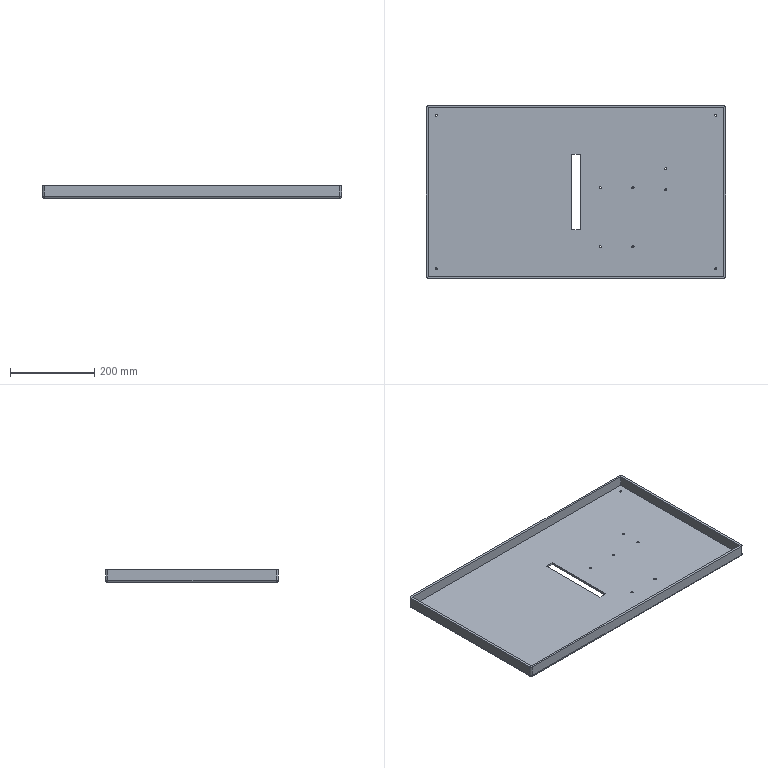Part | SolidWorks | features Cut 1, Extrusion 1, Fillet 1, HoleWzd 1, ICE 1, Shell 1 | 1 solid | 47 faces | box 710 x 410 x 30 mm | volume 1701440 mm3 | cylinder 28 | plane 15 | sphere 4 | commonest cylinder face diameters 5 x20 10 x8
STEP:
#1=CARTESIAN_POINT('',(329.5,-182.,5.));
#2=VERTEX_POINT('',#1);
#3=CARTESIAN_POINT('',(334.5,-182.,5.));
#4=VERTEX_POINT('',#3);
#5=CARTESIAN_POINT('',(332.,-182.,5.));
#6=DIRECTION('',(0.,0.,1.));
#7=DIRECTION('',(1.,0.,0.));
#8=AXIS2_PLACEMENT_3D('',#5,#6,#7);
#9=CIRCLE('',#8,2.5);
#10=EDGE_CURVE('',#2,#4,#9,.T.);
#11=ORIENTED_EDGE('',*,*,#10,.T.);
#12=CARTESIAN_POINT('',(334.5,-182.,0.));
#13=VERTEX_POINT('',#12);
#14=CARTESIAN_POINT('',(334.5,-182.,10.));
#15=DIRECTION('',(0.,0.,-1.));
#16=VECTOR('',#15,1000.);
#17=LINE('',#14,#16);
#18=EDGE_CURVE('',#4,#13,#17,.T.);
#19=ORIENTED_EDGE('',*,*,#18,.T.);
#20=CARTESIAN_POINT('',(329.5,-182.,0.));
#21=VERTEX_POINT('',#20);
#22=CARTESIAN_POINT('',(332.,-182.,0.));
#23=DIRECTION('',(0.,0.,-1.));
#24=DIRECTION('',(1.,0.,0.));
#25=AXIS2_PLACEMENT_3D('',#22,#23,#24);
#26=CIRCLE('',#25,2.5);
#27=EDGE_CURVE('',#13,#21,#26,.T.);
#28=ORIENTED_EDGE('',*,*,#27,.T.);
#29=CARTESIAN_POINT('',(329.5,-182.,10.));
#30=DIRECTION('',(0.,0.,-1.));
#31=VECTOR('',#30,1000.);
#32=LINE('',#29,#31);
#33=EDGE_CURVE('',#2,#21,#32,.T.);
#34=ORIENTED_EDGE('',*,*,#33,.F.);
#35=EDGE_LOOP('',(#11,#19,#28,#34));
#36=FACE_OUTER_BOUND('',#35,.T.);
#37=CARTESIAN_POINT('',(332.,-182.,10.));
#38=DIRECTION('',(0.,0.,-1.));
#39=DIRECTION('',(-1.,0.,0.));
#40=AXIS2_PLACEMENT_3D('',#37,#38,#39);
#41=CYLINDRICAL_SURFACE('',#40,2.5);
#42=ADVANCED_FACE('',(#36),#41,.F.);
#43=CARTESIAN_POINT('',(-334.5,-182.,5.));
#44=VERTEX_POINT('',#43);
#45=CARTESIAN_POINT('',(-329.5,-182.,5.));
#46=VERTEX_POINT('',#45);
#47=CARTESIAN_POINT('',(-332.,-182.,5.));
#48=DIRECTION('',(0.,0.,1.));
#49=DIRECTION('',(1.,0.,0.));
#50=AXIS2_PLACEMENT_3D('',#47,#48,#49);
#51=CIRCLE('',#50,2.5);
#52=EDGE_CURVE('',#44,#46,#51,.T.);
#53=ORIENTED_EDGE('',*,*,#52,.T.);
#54=CARTESIAN_POINT('',(-329.5,-182.,0.));
#55=VERTEX_POINT('',#54);
#56=CARTESIAN_POINT('',(-329.5,-182.,10.));
#57=DIRECTION('',(0.,0.,-1.));
#58=VECTOR('',#57,1000.);
#59=LINE('',#56,#58);
#60=EDGE_CURVE('',#46,#55,#59,.T.);
#61=ORIENTED_EDGE('',*,*,#60,.T.);
#62=CARTESIAN_POINT('',(-334.5,-182.,0.));
#63=VERTEX_POINT('',#62);
#64=CARTESIAN_POINT('',(-332.,-182.,0.));
#65=DIRECTION('',(0.,0.,-1.));
#66=DIRECTION('',(-1.,0.,0.));
#67=AXIS2_PLACEMENT_3D('',#64,#65,#66);
#68=CIRCLE('',#67,2.5);
#69=EDGE_CURVE('',#55,#63,#68,.T.);
#70=ORIENTED_EDGE('',*,*,#69,.T.);
#71=CARTESIAN_POINT('',(-334.5,-182.,10.));
#72=DIRECTION('',(0.,0.,-1.));
#73=VECTOR('',#72,1000.);
#74=LINE('',#71,#73);
#75=EDGE_CURVE('',#44,#63,#74,.T.);
#76=ORIENTED_EDGE('',*,*,#75,.F.);
#77=EDGE_LOOP('',(#53,#61,#70,#76));
#78=FACE_OUTER_BOUND('',#77,.T.);
#79=CARTESIAN_POINT('',(-332.,-182.,10.));
#80=DIRECTION('',(0.,0.,-1.));
#81=DIRECTION('',(-1.,0.,0.));
#82=AXIS2_PLACEMENT_3D('',#79,#80,#81);
#83=CYLINDRICAL_SURFACE('',#82,2.5);
#84=ADVANCED_FACE('',(#78),#83,.F.);
#85=CARTESIAN_POINT('',(-334.5,182.,5.));
#86=VERTEX_POINT('',#85);
#87=CARTESIAN_POINT('',(-329.5,182.,5.));
#88=VERTEX_POINT('',#87);
#89=CARTESIAN_POINT('',(-332.,182.,5.));
#90=DIRECTION('',(0.,0.,1.));
#91=DIRECTION('',(1.,0.,0.));
#92=AXIS2_PLACEMENT_3D('',#89,#90,#91);
#93=CIRCLE('',#92,2.5);
#94=EDGE_CURVE('',#86,#88,#93,.T.);
#95=ORIENTED_EDGE('',*,*,#94,.T.);
#96=CARTESIAN_POINT('',(-329.5,182.,0.));
#97=VERTEX_POINT('',#96);
#98=CARTESIAN_POINT('',(-329.5,182.,10.));
#99=DIRECTION('',(0.,0.,-1.));
#100=VECTOR('',#99,1000.);
#101=LINE('',#98,#100);
#102=EDGE_CURVE('',#88,#97,#101,.T.);
#103=ORIENTED_EDGE('',*,*,#102,.T.);
#104=CARTESIAN_POINT('',(-334.5,182.,0.));
#105=VERTEX_POINT('',#104);
#106=CARTESIAN_POINT('',(-332.,182.,0.));
#107=DIRECTION('',(0.,0.,-1.));
#108=DIRECTION('',(1.,0.,0.));
#109=AXIS2_PLACEMENT_3D('',#106,#107,#108);
#110=CIRCLE('',#109,2.5);
#111=EDGE_CURVE('',#97,#105,#110,.T.);
#112=ORIENTED_EDGE('',*,*,#111,.T.);
#113=CARTESIAN_POINT('',(-334.5,182.,10.));
#114=DIRECTION('',(0.,0.,-1.));
#115=VECTOR('',#114,1000.);
#116=LINE('',#113,#115);
#117=EDGE_CURVE('',#86,#105,#116,.T.);
#118=ORIENTED_EDGE('',*,*,#117,.F.);
#119=EDGE_LOOP('',(#95,#103,#112,#118));
#120=FACE_OUTER_BOUND('',#119,.T.);
#121=CARTESIAN_POINT('',(-332.,182.,10.));
#122=DIRECTION('',(0.,0.,-1.));
#123=DIRECTION('',(-1.,0.,0.));
#124=AXIS2_PLACEMENT_3D('',#121,#122,#123);
#125=CYLINDRICAL_SURFACE('',#124,2.5);
#126=ADVANCED_FACE('',(#120),#125,.F.);
#127=CARTESIAN_POINT('',(329.5,182.,5.));
#128=VERTEX_POINT('',#127);
#129=CARTESIAN_POINT('',(334.5,182.,5.));
#130=VERTEX_POINT('',#129);
#131=CARTESIAN_POINT('',(332.,182.,5.));
#132=DIRECTION('',(0.,0.,1.));
#133=DIRECTION('',(1.,0.,0.));
#134=AXIS2_PLACEMENT_3D('',#131,#132,#133);
#135=CIRCLE('',#134,2.5);
#136=EDGE_CURVE('',#128,#130,#135,.T.);
#137=ORIENTED_EDGE('',*,*,#136,.T.);
#138=CARTESIAN_POINT('',(334.5,182.,0.));
#139=VERTEX_POINT('',#138);
#140=CARTESIAN_POINT('',(334.5,182.,10.));
#141=DIRECTION('',(0.,0.,-1.));
#142=VECTOR('',#141,1000.);
#143=LINE('',#140,#142);
#144=EDGE_CURVE('',#130,#139,#143,.T.);
#145=ORIENTED_EDGE('',*,*,#144,.T.);
#146=CARTESIAN_POINT('',(329.5,182.,0.));
#147=VERTEX_POINT('',#146);
#148=CARTESIAN_POINT('',(332.,182.,0.));
#149=DIRECTION('',(0.,0.,-1.));
#150=DIRECTION('',(-1.,0.,0.));
#151=AXIS2_PLACEMENT_3D('',#148,#149,#150);
#152=CIRCLE('',#151,2.5);
#153=EDGE_CURVE('',#139,#147,#152,.T.);
#154=ORIENTED_EDGE('',*,*,#153,.T.);
#155=CARTESIAN_POINT('',(329.5,182.,10.));
#156=DIRECTION('',(0.,0.,-1.));
#157=VECTOR('',#156,1000.);
#158=LINE('',#155,#157);
#159=EDGE_CURVE('',#128,#147,#158,.T.);
#160=ORIENTED_EDGE('',*,*,#159,.F.);
#161=EDGE_LOOP('',(#137,#145,#154,#160));
#162=FACE_OUTER_BOUND('',#161,.T.);
#163=CARTESIAN_POINT('',(332.,182.,10.));
#164=DIRECTION('',(0.,0.,-1.));
#165=DIRECTION('',(-1.,0.,0.));
#166=AXIS2_PLACEMENT_3D('',#163,#164,#165);
#167=CYLINDRICAL_SURFACE('',#166,2.5);
#168=ADVANCED_FACE('',(#162),#167,.F.);
#169=CARTESIAN_POINT('',(132.625,-130.,5.));
#170=VERTEX_POINT('',#169);
#171=CARTESIAN_POINT('',(137.625,-130.,5.));
#172=VERTEX_POINT('',#171);
#173=CARTESIAN_POINT('',(135.125,-130.,5.));
#174=DIRECTION('',(0.,0.,1.));
#175=DIRECTION('',(1.,0.,0.));
#176=AXIS2_PLACEMENT_3D('',#173,#174,#175);
#177=CIRCLE('',#176,2.5);
#178=EDGE_CURVE('',#170,#172,#177,.T.);
#179=ORIENTED_EDGE('',*,*,#178,.T.);
#180=CARTESIAN_POINT('',(137.625,-130.,0.));
#181=VERTEX_POINT('',#180);
#182=CARTESIAN_POINT('',(137.625,-130.,0.));
#183=DIRECTION('',(0.,0.,-1.));
#184=VECTOR('',#183,1000.);
#185=LINE('',#182,#184);
#186=EDGE_CURVE('',#172,#181,#185,.T.);
#187=ORIENTED_EDGE('',*,*,#186,.T.);
#188=CARTESIAN_POINT('',(132.625,-130.,0.));
#189=VERTEX_POINT('',#188);
#190=CARTESIAN_POINT('',(135.125,-130.,0.));
#191=DIRECTION('',(0.,0.,-1.));
#192=DIRECTION('',(-1.,0.,0.));
#193=AXIS2_PLACEMENT_3D('',#190,#191,#192);
#194=CIRCLE('',#193,2.5);
#195=EDGE_CURVE('',#181,#189,#194,.T.);
#196=ORIENTED_EDGE('',*,*,#195,.T.);
#197=CARTESIAN_POINT('',(132.625,-130.,0.));
#198=DIRECTION('',(0.,0.,-1.));
#199=VECTOR('',#198,1000.);
#200=LINE('',#197,#199);
#201=EDGE_CURVE('',#170,#189,#200,.T.);
#202=ORIENTED_EDGE('',*,*,#201,.F.);
#203=EDGE_LOOP('',(#179,#187,#196,#202));
#204=FACE_OUTER_BOUND('',#203,.T.);
#205=CARTESIAN_POINT('',(135.125,-130.,0.));
#206=DIRECTION('',(0.,0.,-1.));
#207=DIRECTION('',(-1.,0.,0.));
#208=AXIS2_PLACEMENT_3D('',#205,#206,#207);
#209=CYLINDRICAL_SURFACE('',#208,2.5);
#210=ADVANCED_FACE('',(#204),#209,.F.);
#211=CARTESIAN_POINT('',(55.375,-130.,5.));
#212=VERTEX_POINT('',#211);
#213=CARTESIAN_POINT('',(60.375,-130.,5.));
#214=VERTEX_POINT('',#213);
#215=CARTESIAN_POINT('',(57.875,-130.,5.));
#216=DIRECTION('',(0.,0.,1.));
#217=DIRECTION('',(1.,0.,0.));
#218=AXIS2_PLACEMENT_3D('',#215,#216,#217);
#219=CIRCLE('',#218,2.5);
#220=EDGE_CURVE('',#212,#214,#219,.T.);
#221=ORIENTED_EDGE('',*,*,#220,.T.);
#222=CARTESIAN_POINT('',(60.375,-130.,0.));
#223=VERTEX_POINT('',#222);
#224=CARTESIAN_POINT('',(60.375,-130.,0.));
#225=DIRECTION('',(0.,0.,-1.));
#226=VECTOR('',#225,1000.);
#227=LINE('',#224,#226);
#228=EDGE_CURVE('',#214,#223,#227,.T.);
#229=ORIENTED_EDGE('',*,*,#228,.T.);
#230=CARTESIAN_POINT('',(55.375,-130.,0.));
#231=VERTEX_POINT('',#230);
#232=CARTESIAN_POINT('',(57.875,-130.,0.));
#233=DIRECTION('',(0.,0.,-1.));
#234=DIRECTION('',(-1.,0.,0.));
#235=AXIS2_PLACEMENT_3D('',#232,#233,#234);
#236=CIRCLE('',#235,2.5);
#237=EDGE_CURVE('',#223,#231,#236,.T.);
#238=ORIENTED_EDGE('',*,*,#237,.T.);
#239=CARTESIAN_POINT('',(55.375,-130.,0.));
#240=DIRECTION('',(0.,0.,-1.));
#241=VECTOR('',#240,1000.);
#242=LINE('',#239,#241);
#243=EDGE_CURVE('',#212,#231,#242,.T.);
#244=ORIENTED_EDGE('',*,*,#243,.F.);
#245=EDGE_LOOP('',(#221,#229,#238,#244));
#246=FACE_OUTER_BOUND('',#245,.T.);
#247=CARTESIAN_POINT('',(57.875,-130.,0.));
#248=DIRECTION('',(0.,0.,-1.));
#249=DIRECTION('',(-1.,0.,0.));
#250=AXIS2_PLACEMENT_3D('',#247,#248,#249);
#251=CYLINDRICAL_SURFACE('',#250,2.5);
#252=ADVANCED_FACE('',(#246),#251,.F.);
#253=CARTESIAN_POINT('',(210.5,5.,5.));
#254=VERTEX_POINT('',#253);
#255=CARTESIAN_POINT('',(215.5,5.,5.));
#256=VERTEX_POINT('',#255);
#257=CARTESIAN_POINT('',(213.,5.,5.));
#258=DIRECTION('',(0.,0.,1.));
#259=DIRECTION('',(1.,0.,0.));
#260=AXIS2_PLACEMENT_3D('',#257,#258,#259);
#261=CIRCLE('',#260,2.5);
#262=EDGE_CURVE('',#254,#256,#261,.T.);
#263=ORIENTED_EDGE('',*,*,#262,.T.);
#264=CARTESIAN_POINT('',(215.5,5.,0.));
#265=VERTEX_POINT('',#264);
#266=CARTESIAN_POINT('',(215.5,5.,0.));
#267=DIRECTION('',(0.,0.,-1.));
#268=VECTOR('',#267,1000.);
#269=LINE('',#266,#268);
#270=EDGE_CURVE('',#256,#265,#269,.T.);
#271=ORIENTED_EDGE('',*,*,#270,.T.);
#272=CARTESIAN_POINT('',(210.5,5.,0.));
#273=VERTEX_POINT('',#272);
#274=CARTESIAN_POINT('',(213.,5.,0.));
#275=DIRECTION('',(0.,0.,-1.));
#276=DIRECTION('',(-1.,0.,0.));
#277=AXIS2_PLACEMENT_3D('',#274,#275,#276);
#278=CIRCLE('',#277,2.5);
#279=EDGE_CURVE('',#265,#273,#278,.T.);
#280=ORIENTED_EDGE('',*,*,#279,.T.);
#281=CARTESIAN_POINT('',(210.5,5.,0.));
#282=DIRECTION('',(0.,0.,-1.));
#283=VECTOR('',#282,1000.);
#284=LINE('',#281,#283);
#285=EDGE_CURVE('',#254,#273,#284,.T.);
#286=ORIENTED_EDGE('',*,*,#285,.F.);
#287=EDGE_LOOP('',(#263,#271,#280,#286));
#288=FACE_OUTER_BOUND('',#287,.T.);
#289=CARTESIAN_POINT('',(213.,5.,0.));
#290=DIRECTION('',(0.,0.,-1.));
#291=DIRECTION('',(-1.,0.,0.));
#292=AXIS2_PLACEMENT_3D('',#289,#290,#291);
#293=CYLINDRICAL_SURFACE('',#292,2.5);
#294=ADVANCED_FACE('',(#288),#293,.F.);
#295=CARTESIAN_POINT('',(210.5,55.,5.));
#296=VERTEX_POINT('',#295);
#297=CARTESIAN_POINT('',(215.5,55.,5.));
#298=VERTEX_POINT('',#297);
#299=CARTESIAN_POINT('',(213.,55.,5.));
#300=DIRECTION('',(0.,0.,1.));
#301=DIRECTION('',(1.,0.,0.));
#302=AXIS2_PLACEMENT_3D('',#299,#300,#301);
#303=CIRCLE('',#302,2.5);
#304=EDGE_CURVE('',#296,#298,#303,.T.);
#305=ORIENTED_EDGE('',*,*,#304,.T.);
#306=CARTESIAN_POINT('',(215.5,55.,0.));
#307=VERTEX_POINT('',#306);
#308=CARTESIAN_POINT('',(215.5,55.,0.));
#309=DIRECTION('',(0.,0.,-1.));
#310=VECTOR('',#309,1000.);
#311=LINE('',#308,#310);
#312=EDGE_CURVE('',#298,#307,#311,.T.);
#313=ORIENTED_EDGE('',*,*,#312,.T.);
#314=CARTESIAN_POINT('',(210.5,55.,0.));
#315=VERTEX_POINT('',#314);
#316=CARTESIAN_POINT('',(213.,55.,0.));
#317=DIRECTION('',(0.,0.,-1.));
#318=DIRECTION('',(-1.,0.,0.));
#319=AXIS2_PLACEMENT_3D('',#316,#317,#318);
#320=CIRCLE('',#319,2.5);
#321=EDGE_CURVE('',#307,#315,#320,.T.);
#322=ORIENTED_EDGE('',*,*,#321,.T.);
#323=CARTESIAN_POINT('',(210.5,55.,0.));
#324=DIRECTION('',(0.,0.,-1.));
#325=VECTOR('',#324,1000.);
#326=LINE('',#323,#325);
#327=EDGE_CURVE('',#296,#315,#326,.T.);
#328=ORIENTED_EDGE('',*,*,#327,.F.);
#329=EDGE_LOOP('',(#305,#313,#322,#328));
#330=FACE_OUTER_BOUND('',#329,.T.);
#331=CARTESIAN_POINT('',(213.,55.,0.));
#332=DIRECTION('',(0.,0.,-1.));
#333=DIRECTION('',(-1.,0.,0.));
#334=AXIS2_PLACEMENT_3D('',#331,#332,#333);
#335=CYLINDRICAL_SURFACE('',#334,2.5);
#336=ADVANCED_FACE('',(#330),#335,.F.);
#337=CARTESIAN_POINT('',(132.625,10.,5.));
#338=VERTEX_POINT('',#337);
#339=CARTESIAN_POINT('',(137.625,10.,5.));
#340=VERTEX_POINT('',#339);
#341=CARTESIAN_POINT('',(135.125,10.,5.));
#342=DIRECTION('',(0.,0.,1.));
#343=DIRECTION('',(1.,0.,0.));
#344=AXIS2_PLACEMENT_3D('',#341,#342,#343);
#345=CIRCLE('',#344,2.5);
#346=EDGE_CURVE('',#338,#340,#345,.T.);
#347=ORIENTED_EDGE('',*,*,#346,.T.);
#348=CARTESIAN_POINT('',(137.625,10.,0.));
#349=VERTEX_POINT('',#348);
#350=CARTESIAN_POINT('',(137.625,10.,0.));
#351=DIRECTION('',(0.,0.,-1.));
#352=VECTOR('',#351,1000.);
#353=LINE('',#350,#352);
#354=EDGE_CURVE('',#340,#349,#353,.T.);
#355=ORIENTED_EDGE('',*,*,#354,.T.);
#356=CARTESIAN_POINT('',(132.625,10.,0.));
#357=VERTEX_POINT('',#356);
#358=CARTESIAN_POINT('',(135.125,10.,0.));
#359=DIRECTION('',(0.,0.,-1.));
#360=DIRECTION('',(-1.,0.,0.));
#361=AXIS2_PLACEMENT_3D('',#358,#359,#360);
#362=CIRCLE('',#361,2.5);
#363=EDGE_CURVE('',#349,#357,#362,.T.);
#364=ORIENTED_EDGE('',*,*,#363,.T.);
#365=CARTESIAN_POINT('',(132.625,10.,0.));
#366=DIRECTION('',(0.,0.,-1.));
#367=VECTOR('',#366,1000.);
#368=LINE('',#365,#367);
#369=EDGE_CURVE('',#338,#357,#368,.T.);
#370=ORIENTED_EDGE('',*,*,#369,.F.);
#371=EDGE_LOOP('',(#347,#355,#364,#370));
#372=FACE_OUTER_BOUND('',#371,.T.);
#373=CARTESIAN_POINT('',(135.125,10.,0.));
#374=DIRECTION('',(0.,0.,-1.));
#375=DIRECTION('',(-1.,0.,0.));
#376=AXIS2_PLACEMENT_3D('',#373,#374,#375);
#377=CYLINDRICAL_SURFACE('',#376,2.5);
#378=ADVANCED_FACE('',(#372),#377,.F.);
#379=CARTESIAN_POINT('',(55.375,10.,5.));
#380=VERTEX_POINT('',#379);
#381=CARTESIAN_POINT('',(60.375,10.,5.));
#382=VERTEX_POINT('',#381);
#383=CARTESIAN_POINT('',(57.875,10.,5.));
#384=DIRECTION('',(0.,0.,1.));
#385=DIRECTION('',(1.,0.,0.));
#386=AXIS2_PLACEMENT_3D('',#383,#384,#385);
#387=CIRCLE('',#386,2.5);
#388=EDGE_CURVE('',#380,#382,#387,.T.);
#389=ORIENTED_EDGE('',*,*,#388,.T.);
#390=CARTESIAN_POINT('',(60.375,10.,0.));
#391=VERTEX_POINT('',#390);
#392=CARTESIAN_POINT('',(60.375,10.,0.));
#393=DIRECTION('',(0.,0.,-1.));
#394=VECTOR('',#393,1000.);
#395=LINE('',#392,#394);
#396=EDGE_CURVE('',#382,#391,#395,.T.);
#397=ORIENTED_EDGE('',*,*,#396,.T.);
#398=CARTESIAN_POINT('',(55.375,10.,0.));
#399=VERTEX_POINT('',#398);
#400=CARTESIAN_POINT('',(57.875,10.,0.));
#401=DIRECTION('',(0.,0.,-1.));
#402=DIRECTION('',(-1.,0.,0.));
#403=AXIS2_PLACEMENT_3D('',#400,#401,#402);
#404=CIRCLE('',#403,2.5);
#405=EDGE_CURVE('',#391,#399,#404,.T.);
#406=ORIENTED_EDGE('',*,*,#405,.T.);
#407=CARTESIAN_POINT('',(55.375,10.,0.));
#408=DIRECTION('',(0.,0.,-1.));
#409=VECTOR('',#408,1000.);
#410=LINE('',#407,#409);
#411=EDGE_CURVE('',#380,#399,#410,.T.);
#412=ORIENTED_EDGE('',*,*,#411,.F.);
#413=EDGE_LOOP('',(#389,#397,#406,#412));
#414=FACE_OUTER_BOUND('',#413,.T.);
#415=CARTESIAN_POINT('',(57.875,10.,0.));
#416=DIRECTION('',(0.,0.,-1.));
#417=DIRECTION('',(-1.,0.,0.));
#418=AXIS2_PLACEMENT_3D('',#415,#416,#417);
#419=CYLINDRICAL_SURFACE('',#418,2.5);
#420=ADVANCED_FACE('',(#414),#419,.F.);
#421=CARTESIAN_POINT('',(355.,-200.,30.));
#422=VERTEX_POINT('',#421);
#423=CARTESIAN_POINT('',(355.,200.,30.));
#424=VERTEX_POINT('',#423);
#425=CARTESIAN_POINT('',(355.,205.,30.));
#426=DIRECTION('',(0.,1.,0.));
#427=VECTOR('',#426,1000.);
#428=LINE('',#425,#427);
#429=EDGE_CURVE('',#422,#424,#428,.T.);
#430=ORIENTED_EDGE('',*,*,#429,.F.);
#431=CARTESIAN_POINT('',(355.,-200.,5.));
#432=VERTEX_POINT('',#431);
#433=CARTESIAN_POINT('',(355.,-200.,30.));
#434=DIRECTION('',(0.,0.,-1.));
#435=VECTOR('',#434,1000.);
#436=LINE('',#433,#435);
#437=EDGE_CURVE('',#422,#432,#436,.T.);
#438=ORIENTED_EDGE('',*,*,#437,.T.);
#439=CARTESIAN_POINT('',(355.,200.,5.));
#440=VERTEX_POINT('',#439);
#441=CARTESIAN_POINT('',(355.,205.,5.));
#442=DIRECTION('',(0.,1.,0.));
#443=VECTOR('',#442,1000.);
#444=LINE('',#441,#443);
#445=EDGE_CURVE('',#432,#440,#444,.T.);
#446=ORIENTED_EDGE('',*,*,#445,.T.);
#447=CARTESIAN_POINT('',(355.,200.,30.));
#448=DIRECTION('',(0.,0.,1.));
#449=VECTOR('',#448,1000.);
#450=LINE('',#447,#449);
#451=EDGE_CURVE('',#440,#424,#450,.T.);
#452=ORIENTED_EDGE('',*,*,#451,.T.);
#453=EDGE_LOOP('',(#430,#438,#446,#452));
#454=FACE_OUTER_BOUND('',#453,.T.);
#455=CARTESIAN_POINT('',(355.,205.,30.));
#456=DIRECTION('',(-1.,0.,0.));
#457=DIRECTION('',(0.,0.,1.));
#458=AXIS2_PLACEMENT_3D('',#455,#456,#457);
#459=PLANE('',#458);
#460=ADVANCED_FACE('',(#454),#459,.F.);
#461=CARTESIAN_POINT('',(350.,205.,30.));
#462=VERTEX_POINT('',#461);
#463=CARTESIAN_POINT('',(-350.,205.,30.));
#464=VERTEX_POINT('',#463);
#465=CARTESIAN_POINT('',(-355.,205.,30.));
#466=DIRECTION('',(-1.,0.,0.));
#467=VECTOR('',#466,1000.);
#468=LINE('',#465,#467);
#469=EDGE_CURVE('',#462,#464,#468,.T.);
#470=ORIENTED_EDGE('',*,*,#469,.F.);
#471=CARTESIAN_POINT('',(350.,205.,5.));
#472=VERTEX_POINT('',#471);
#473=CARTESIAN_POINT('',(350.,205.,30.));
#474=DIRECTION('',(0.,0.,-1.));
#475=VECTOR('',#474,1000.);
#476=LINE('',#473,#475);
#477=EDGE_CURVE('',#462,#472,#476,.T.);
#478=ORIENTED_EDGE('',*,*,#477,.T.);
#479=CARTESIAN_POINT('',(-350.,205.,5.));
#480=VERTEX_POINT('',#479);
#481=CARTESIAN_POINT('',(-355.,205.,5.));
#482=DIRECTION('',(-1.,0.,0.));
#483=VECTOR('',#482,1000.);
#484=LINE('',#481,#483);
#485=EDGE_CURVE('',#472,#480,#484,.T.);
#486=ORIENTED_EDGE('',*,*,#485,.T.);
#487=CARTESIAN_POINT('',(-350.,205.,30.));
#488=DIRECTION('',(0.,0.,1.));
#489=VECTOR('',#488,1000.);
#490=LINE('',#487,#489);
#491=EDGE_CURVE('',#480,#464,#490,.T.);
#492=ORIENTED_EDGE('',*,*,#491,.T.);
#493=EDGE_LOOP('',(#470,#478,#486,#492));
#494=FACE_OUTER_BOUND('',#493,.T.);
#495=CARTESIAN_POINT('',(-355.,205.,30.));
#496=DIRECTION('',(0.,-1.,0.));
#497=DIRECTION('',(0.,0.,-1.));
#498=AXIS2_PLACEMENT_3D('',#495,#496,#497);
#499=PLANE('',#498);
#500=ADVANCED_FACE('',(#494),#499,.F.);
#501=CARTESIAN_POINT('',(-355.,200.,5.));
#502=VERTEX_POINT('',#501);
#503=CARTESIAN_POINT('',(-355.,-200.,5.));
#504=VERTEX_POINT('',#503);
#505=CARTESIAN_POINT('',(-355.,205.,5.));
#506=DIRECTION('',(0.,-1.,0.));
#507=VECTOR('',#506,1000.);
#508=LINE('',#505,#507);
#509=EDGE_CURVE('',#502,#504,#508,.T.);
#510=ORIENTED_EDGE('',*,*,#509,.T.);
#511=CARTESIAN_POINT('',(-355.,-200.,30.));
#512=VERTEX_POINT('',#511);
#513=CARTESIAN_POINT('',(-355.,-200.,30.));
#514=DIRECTION('',(0.,0.,1.));
#515=VECTOR('',#514,1000.);
#516=LINE('',#513,#515);
#517=EDGE_CURVE('',#504,#512,#516,.T.);
#518=ORIENTED_EDGE('',*,*,#517,.T.);
#519=CARTESIAN_POINT('',(-355.,200.,30.));
#520=VERTEX_POINT('',#519);
#521=CARTESIAN_POINT('',(-355.,205.,30.));
#522=DIRECTION('',(0.,-1.,0.));
#523=VECTOR('',#522,1000.);
#524=LINE('',#521,#523);
#525=EDGE_CURVE('',#520,#512,#524,.T.);
#526=ORIENTED_EDGE('',*,*,#525,.F.);
#527=CARTESIAN_POINT('',(-355.,200.,30.));
#528=DIRECTION('',(0.,0.,-1.));
#529=VECTOR('',#528,1000.);
#530=LINE('',#527,#529);
#531=EDGE_CURVE('',#520,#502,#530,.T.);
#532=ORIENTED_EDGE('',*,*,#531,.T.);
#533=EDGE_LOOP('',(#510,#518,#526,#532));
#534=FACE_OUTER_BOUND('',#533,.T.);
#535=CARTESIAN_POINT('',(-355.,205.,30.));
#536=DIRECTION('',(1.,0.,0.));
#537=DIRECTION('',(0.,1.,0.));
#538=AXIS2_PLACEMENT_3D('',#535,#536,#537);
#539=PLANE('',#538);
#540=ADVANCED_FACE('',(#534),#539,.F.);
#541=CARTESIAN_POINT('',(-350.,-205.,30.));
#542=VERTEX_POINT('',#541);
#543=CARTESIAN_POINT('',(350.,-205.,30.));
#544=VERTEX_POINT('',#543);
#545=CARTESIAN_POINT('',(-355.,-205.,30.));
#546=DIRECTION('',(1.,0.,0.));
#547=VECTOR('',#546,1000.);
#548=LINE('',#545,#547);
#549=EDGE_CURVE('',#542,#544,#548,.T.);
#550=ORIENTED_EDGE('',*,*,#549,.F.);
#551=CARTESIAN_POINT('',(-350.,-205.,5.));
#552=VERTEX_POINT('',#551);
#553=CARTESIAN_POINT('',(-350.,-205.,30.));
#554=DIRECTION('',(0.,0.,-1.));
#555=VECTOR('',#554,1000.);
#556=LINE('',#553,#555);
#557=EDGE_CURVE('',#542,#552,#556,.T.);
#558=ORIENTED_EDGE('',*,*,#557,.T.);
#559=CARTESIAN_POINT('',(350.,-205.,5.));
#560=VERTEX_POINT('',#559);
#561=CARTESIAN_POINT('',(-355.,-205.,5.));
#562=DIRECTION('',(1.,0.,0.));
#563=VECTOR('',#562,1000.);
#564=LINE('',#561,#563);
#565=EDGE_CURVE('',#552,#560,#564,.T.);
#566=ORIENTED_EDGE('',*,*,#565,.T.);
#567=CARTESIAN_POINT('',(350.,-205.,30.));
#568=DIRECTION('',(0.,0.,1.));
#569=VECTOR('',#568,1000.);
#570=LINE('',#567,#569);
#571=EDGE_CURVE('',#560,#544,#570,.T.);
#572=ORIENTED_EDGE('',*,*,#571,.T.);
#573=EDGE_LOOP('',(#550,#558,#566,#572));
#574=FACE_OUTER_BOUND('',#573,.T.);
#575=CARTESIAN_POINT('',(-355.,-205.,30.));
#576=DIRECTION('',(0.,1.,0.));
#577=DIRECTION('',(0.,0.,1.));
#578=AXIS2_PLACEMENT_3D('',#575,#576,#577);
#579=PLANE('',#578);
#580=ADVANCED_FACE('',(#574),#579,.F.);
#581=CARTESIAN_POINT('',(-350.,200.,30.));
#582=VERTEX_POINT('',#581);
#583=CARTESIAN_POINT('',(-350.,-200.,30.));
#584=VERTEX_POINT('',#583);
#585=CARTESIAN_POINT('',(-350.,205.,30.));
#586=DIRECTION('',(0.,-1.,0.));
#587=VECTOR('',#586,1000.);
#588=LINE('',#585,#587);
#589=EDGE_CURVE('',#582,#584,#588,.T.);
#590=ORIENTED_EDGE('',*,*,#589,.F.);
#591=CARTESIAN_POINT('',(350.,200.,30.));
#592=VERTEX_POINT('',#591);
#593=CARTESIAN_POINT('',(-355.,200.,30.));
#594=DIRECTION('',(-1.,0.,0.));
#595=VECTOR('',#594,1000.);
#596=LINE('',#593,#595);
#597=EDGE_CURVE('',#592,#582,#596,.T.);
#598=ORIENTED_EDGE('',*,*,#597,.F.);
#599=CARTESIAN_POINT('',(350.,-200.,30.));
#600=VERTEX_POINT('',#599);
#601=CARTESIAN_POINT('',(350.,205.,30.));
#602=DIRECTION('',(0.,1.,0.));
#603=VECTOR('',#602,1000.);
#604=LINE('',#601,#603);
#605=EDGE_CURVE('',#600,#592,#604,.T.);
#606=ORIENTED_EDGE('',*,*,#605,.F.);
#607=CARTESIAN_POINT('',(-355.,-200.,30.));
#608=DIRECTION('',(1.,0.,0.));
#609=VECTOR('',#608,1000.);
#610=LINE('',#607,#609);
#611=EDGE_CURVE('',#584,#600,#610,.T.);
#612=ORIENTED_EDGE('',*,*,#611,.F.);
#613=EDGE_LOOP('',(#590,#598,#606,#612));
#614=FACE_BOUND('',#613,.T.);
#615=ORIENTED_EDGE('',*,*,#525,.T.);
#616=CARTESIAN_POINT('',(-350.,-200.,30.));
#617=DIRECTION('',(0.,0.,1.));
#618=DIRECTION('',(1.,0.,0.));
#619=AXIS2_PLACEMENT_3D('',#616,#617,#618);
#620=CIRCLE('',#619,5.);
#621=EDGE_CURVE('',#512,#542,#620,.T.);
#622=ORIENTED_EDGE('',*,*,#621,.T.);
#623=ORIENTED_EDGE('',*,*,#549,.T.);
#624=CARTESIAN_POINT('',(350.,-200.,30.));
#625=DIRECTION('',(0.,0.,1.));
#626=DIRECTION('',(1.,0.,0.));
#627=AXIS2_PLACEMENT_3D('',#624,#625,#626);
#628=CIRCLE('',#627,5.);
#629=EDGE_CURVE('',#544,#422,#628,.T.);
#630=ORIENTED_EDGE('',*,*,#629,.T.);
#631=ORIENTED_EDGE('',*,*,#429,.T.);
#632=CARTESIAN_POINT('',(350.,200.,30.));
#633=DIRECTION('',(0.,0.,1.));
#634=DIRECTION('',(1.,0.,0.));
#635=AXIS2_PLACEMENT_3D('',#632,#633,#634);
#636=CIRCLE('',#635,5.);
#637=EDGE_CURVE('',#424,#462,#636,.T.);
#638=ORIENTED_EDGE('',*,*,#637,.T.);
#639=ORIENTED_EDGE('',*,*,#469,.T.);
#640=CARTESIAN_POINT('',(-350.,200.,30.));
#641=DIRECTION('',(0.,0.,1.));
#642=DIRECTION('',(1.,0.,0.));
#643=AXIS2_PLACEMENT_3D('',#640,#641,#642);
#644=CIRCLE('',#643,5.);
#645=EDGE_CURVE('',#464,#520,#644,.T.);
#646=ORIENTED_EDGE('',*,*,#645,.T.);
#647=EDGE_LOOP('',(#615,#622,#623,#630,#631,#638,#639,#646));
#648=FACE_OUTER_BOUND('',#647,.T.);
#649=CARTESIAN_POINT('',(0.,0.,30.));
#650=DIRECTION('',(0.,0.,1.));
#651=DIRECTION('',(1.,0.,0.));
#652=AXIS2_PLACEMENT_3D('',#649,#650,#651);
#653=PLANE('',#652);
#654=ADVANCED_FACE('',(#614,#648),#653,.T.);
#655=CARTESIAN_POINT('',(332.,-182.,0.));
#656=DIRECTION('',(0.,0.,-1.));
#657=DIRECTION('',(1.,0.,0.));
#658=AXIS2_PLACEMENT_3D('',#655,#656,#657);
#659=CIRCLE('',#658,2.5);
#660=EDGE_CURVE('',#21,#13,#659,.T.);
#661=ORIENTED_EDGE('',*,*,#660,.F.);
#662=ORIENTED_EDGE('',*,*,#27,.F.);
#663=EDGE_LOOP('',(#661,#662));
#664=FACE_BOUND('',#663,.T.);
#665=CARTESIAN_POINT('',(-332.,-182.,0.));
#666=DIRECTION('',(0.,0.,-1.));
#667=DIRECTION('',(-1.,0.,0.));
#668=AXIS2_PLACEMENT_3D('',#665,#666,#667);
#669=CIRCLE('',#668,2.5);
#670=EDGE_CURVE('',#63,#55,#669,.T.);
#671=ORIENTED_EDGE('',*,*,#670,.F.);
#672=ORIENTED_EDGE('',*,*,#69,.F.);
#673=EDGE_LOOP('',(#671,#672));
#674=FACE_BOUND('',#673,.T.);
#675=CARTESIAN_POINT('',(-332.,182.,0.));
#676=DIRECTION('',(0.,0.,-1.));
#677=DIRECTION('',(1.,0.,0.));
#678=AXIS2_PLACEMENT_3D('',#675,#676,#677);
#679=CIRCLE('',#678,2.5);
#680=EDGE_CURVE('',#105,#97,#679,.T.);
#681=ORIENTED_EDGE('',*,*,#680,.F.);
#682=ORIENTED_EDGE('',*,*,#111,.F.);
#683=EDGE_LOOP('',(#681,#682));
#684=FACE_BOUND('',#683,.T.);
#685=CARTESIAN_POINT('',(332.,182.,0.));
#686=DIRECTION('',(0.,0.,-1.));
#687=DIRECTION('',(-1.,0.,0.));
#688=AXIS2_PLACEMENT_3D('',#685,#686,#687);
#689=CIRCLE('',#688,2.5);
#690=EDGE_CURVE('',#147,#139,#689,.T.);
#691=ORIENTED_EDGE('',*,*,#690,.F.);
#692=ORIENTED_EDGE('',*,*,#153,.F.);
#693=EDGE_LOOP('',(#691,#692));
#694=FACE_BOUND('',#693,.T.);
#695=CARTESIAN_POINT('',(135.125,-130.,0.));
#696=DIRECTION('',(0.,0.,-1.));
#697=DIRECTION('',(-1.,0.,0.));
#698=AXIS2_PLACEMENT_3D('',#695,#696,#697);
#699=CIRCLE('',#698,2.5);
#700=EDGE_CURVE('',#189,#181,#699,.T.);
#701=ORIENTED_EDGE('',*,*,#700,.F.);
#702=ORIENTED_EDGE('',*,*,#195,.F.);
#703=EDGE_LOOP('',(#701,#702));
#704=FACE_BOUND('',#703,.T.);
#705=CARTESIAN_POINT('',(57.875,-130.,0.));
#706=DIRECTION('',(0.,0.,-1.));
#707=DIRECTION('',(-1.,0.,0.));
#708=AXIS2_PLACEMENT_3D('',#705,#706,#707);
#709=CIRCLE('',#708,2.5);
#710=EDGE_CURVE('',#231,#223,#709,.T.);
#711=ORIENTED_EDGE('',*,*,#710,.F.);
#712=ORIENTED_EDGE('',*,*,#237,.F.);
#713=EDGE_LOOP('',(#711,#712));
#714=FACE_BOUND('',#713,.T.);
#715=CARTESIAN_POINT('',(213.,5.,0.));
#716=DIRECTION('',(0.,0.,-1.));
#717=DIRECTION('',(-1.,0.,0.));
#718=AXIS2_PLACEMENT_3D('',#715,#716,#717);
#719=CIRCLE('',#718,2.5);
#720=EDGE_CURVE('',#273,#265,#719,.T.);
#721=ORIENTED_EDGE('',*,*,#720,.F.);
#722=ORIENTED_EDGE('',*,*,#279,.F.);
#723=EDGE_LOOP('',(#721,#722));
#724=FACE_BOUND('',#723,.T.);
#725=CARTESIAN_POINT('',(213.,55.,0.));
#726=DIRECTION('',(0.,0.,-1.));
#727=DIRECTION('',(-1.,0.,0.));
#728=AXIS2_PLACEMENT_3D('',#725,#726,#727);
#729=CIRCLE('',#728,2.5);
#730=EDGE_CURVE('',#315,#307,#729,.T.);
#731=ORIENTED_EDGE('',*,*,#730,.F.);
#732=ORIENTED_EDGE('',*,*,#321,.F.);
#733=EDGE_LOOP('',(#731,#732));
#734=FACE_BOUND('',#733,.T.);
#735=CARTESIAN_POINT('',(135.125,10.,0.));
#736=DIRECTION('',(0.,0.,-1.));
#737=DIRECTION('',(-1.,0.,0.));
#738=AXIS2_PLACEMENT_3D('',#735,#736,#737);
#739=CIRCLE('',#738,2.5);
#740=EDGE_CURVE('',#357,#349,#739,.T.);
#741=ORIENTED_EDGE('',*,*,#740,.F.);
#742=ORIENTED_EDGE('',*,*,#363,.F.);
#743=EDGE_LOOP('',(#741,#742));
#744=FACE_BOUND('',#743,.T.);
#745=CARTESIAN_POINT('',(57.875,10.,0.));
#746=DIRECTION('',(0.,0.,-1.));
#747=DIRECTION('',(-1.,0.,0.));
#748=AXIS2_PLACEMENT_3D('',#745,#746,#747);
#749=CIRCLE('',#748,2.5);
#750=EDGE_CURVE('',#399,#391,#749,.T.);
#751=ORIENTED_EDGE('',*,*,#750,.F.);
#752=ORIENTED_EDGE('',*,*,#405,.F.);
#753=EDGE_LOOP('',(#751,#752));
#754=FACE_BOUND('',#753,.T.);
#755=CARTESIAN_POINT('',(-10.,90.,0.));
#756=VERTEX_POINT('',#755);
#757=CARTESIAN_POINT('',(10.,90.,0.));
#758=VERTEX_POINT('',#757);
#759=CARTESIAN_POINT('',(10.,90.,0.));
#760=DIRECTION('',(1.,0.,0.));
#761=VECTOR('',#760,1000.);
#762=LINE('',#759,#761);
#763=EDGE_CURVE('',#756,#758,#762,.T.);
#764=ORIENTED_EDGE('',*,*,#763,.F.);
#765=CARTESIAN_POINT('',(-10.,-90.,0.));
#766=VERTEX_POINT('',#765);
#767=CARTESIAN_POINT('',(-10.,90.,0.));
#768=DIRECTION('',(0.,1.,0.));
#769=VECTOR('',#768,1000.);
#770=LINE('',#767,#769);
#771=EDGE_CURVE('',#766,#756,#770,.T.);
#772=ORIENTED_EDGE('',*,*,#771,.F.);
#773=CARTESIAN_POINT('',(10.,-90.,0.));
#774=VERTEX_POINT('',#773);
#775=CARTESIAN_POINT('',(10.,-90.,0.));
#776=DIRECTION('',(-1.,0.,0.));
#777=VECTOR('',#776,1000.);
#778=LINE('',#775,#777);
#779=EDGE_CURVE('',#774,#766,#778,.T.);
#780=ORIENTED_EDGE('',*,*,#779,.F.);
#781=CARTESIAN_POINT('',(10.,90.,0.));
#782=DIRECTION('',(0.,-1.,0.));
#783=VECTOR('',#782,1000.);
#784=LINE('',#781,#783);
#785=EDGE_CURVE('',#758,#774,#784,.T.);
#786=ORIENTED_EDGE('',*,*,#785,.F.);
#787=EDGE_LOOP('',(#764,#772,#780,#786));
#788=FACE_BOUND('',#787,.T.);
#789=CARTESIAN_POINT('',(350.,-200.,0.));
#790=VERTEX_POINT('',#789);
#791=CARTESIAN_POINT('',(-350.,-200.,0.));
#792=VERTEX_POINT('',#791);
#793=CARTESIAN_POINT('',(0.,-200.,0.));
#794=DIRECTION('',(-1.,0.,0.));
#795=VECTOR('',#794,1000.);
#796=LINE('',#793,#795);
#797=EDGE_CURVE('',#790,#792,#796,.T.);
#798=ORIENTED_EDGE('',*,*,#797,.T.);
#799=CARTESIAN_POINT('',(-350.,200.,0.));
#800=VERTEX_POINT('',#799);
#801=CARTESIAN_POINT('',(-350.,0.,0.));
#802=DIRECTION('',(0.,1.,0.));
#803=VECTOR('',#802,1000.);
#804=LINE('',#801,#803);
#805=EDGE_CURVE('',#792,#800,#804,.T.);
#806=ORIENTED_EDGE('',*,*,#805,.T.);
#807=CARTESIAN_POINT('',(350.,200.,0.));
#808=VERTEX_POINT('',#807);
#809=CARTESIAN_POINT('',(0.,200.,0.));
#810=DIRECTION('',(1.,0.,0.));
#811=VECTOR('',#810,1000.);
#812=LINE('',#809,#811);
#813=EDGE_CURVE('',#800,#808,#812,.T.);
#814=ORIENTED_EDGE('',*,*,#813,.T.);
#815=CARTESIAN_POINT('',(350.,0.,0.));
#816=DIRECTION('',(0.,-1.,0.));
#817=VECTOR('',#816,1000.);
#818=LINE('',#815,#817);
#819=EDGE_CURVE('',#808,#790,#818,.T.);
#820=ORIENTED_EDGE('',*,*,#819,.T.);
#821=EDGE_LOOP('',(#798,#806,#814,#820));
#822=FACE_OUTER_BOUND('',#821,.T.);
#823=CARTESIAN_POINT('',(0.,0.,0.));
#824=DIRECTION('',(0.,0.,1.));
#825=DIRECTION('',(1.,0.,0.));
#826=AXIS2_PLACEMENT_3D('',#823,#824,#825);
#827=PLANE('',#826);
#828=ADVANCED_FACE('',(#664,#674,#684,#694,#704,#714,#724,#734,#744,#754,#788,#822),#827,.F.);
#829=CARTESIAN_POINT('',(350.,200.,5.));
#830=DIRECTION('',(0.,0.,-1.));
#831=DIRECTION('',(-1.,0.,0.));
#832=AXIS2_PLACEMENT_3D('',#829,#830,#831);
#833=CIRCLE('',#832,5.);
#834=EDGE_CURVE('',#472,#440,#833,.T.);
#835=ORIENTED_EDGE('',*,*,#834,.F.);
#836=ORIENTED_EDGE('',*,*,#477,.F.);
#837=ORIENTED_EDGE('',*,*,#637,.F.);
#838=ORIENTED_EDGE('',*,*,#451,.F.);
#839=EDGE_LOOP('',(#835,#836,#837,#838));
#840=FACE_OUTER_BOUND('',#839,.T.);
#841=CARTESIAN_POINT('',(350.,200.,30.));
#842=DIRECTION('',(0.,0.,-1.));
#843=DIRECTION('',(-1.,0.,0.));
#844=AXIS2_PLACEMENT_3D('',#841,#842,#843);
#845=CYLINDRICAL_SURFACE('',#844,5.);
#846=ADVANCED_FACE('',(#840),#845,.T.);
#847=CARTESIAN_POINT('',(350.,200.,5.));
#848=DIRECTION('',(-1.,0.,0.));
#849=DIRECTION('',(0.,0.,-1.));
#850=AXIS2_PLACEMENT_3D('',#847,#848,#849);
#851=CIRCLE('',#850,5.);
#852=EDGE_CURVE('',#472,#808,#851,.T.);
#853=ORIENTED_EDGE('',*,*,#852,.F.);
#854=ORIENTED_EDGE('',*,*,#834,.T.);
#855=CARTESIAN_POINT('',(350.,200.,5.));
#856=DIRECTION('',(0.,-1.,0.));
#857=DIRECTION('',(0.,0.,1.));
#858=AXIS2_PLACEMENT_3D('',#855,#856,#857);
#859=CIRCLE('',#858,5.);
#860=EDGE_CURVE('',#808,#440,#859,.T.);
#861=ORIENTED_EDGE('',*,*,#860,.F.);
#862=EDGE_LOOP('',(#853,#854,#861));
#863=FACE_OUTER_BOUND('',#862,.T.);
#864=CARTESIAN_POINT('',(350.,200.,5.));
#865=DIRECTION('',(0.,1.,0.));
#866=DIRECTION('',(1.,0.,0.));
#867=AXIS2_PLACEMENT_3D('',#864,#865,#866);
#868=SPHERICAL_SURFACE('',#867,5.);
#869=ADVANCED_FACE('',(#863),#868,.T.);
#870=ORIENTED_EDGE('',*,*,#629,.F.);
#871=ORIENTED_EDGE('',*,*,#571,.F.);
#872=CARTESIAN_POINT('',(350.,-200.,5.));
#873=DIRECTION('',(0.,0.,-1.));
#874=DIRECTION('',(-1.,0.,0.));
#875=AXIS2_PLACEMENT_3D('',#872,#873,#874);
#876=CIRCLE('',#875,5.);
#877=EDGE_CURVE('',#432,#560,#876,.T.);
#878=ORIENTED_EDGE('',*,*,#877,.F.);
#879=ORIENTED_EDGE('',*,*,#437,.F.);
#880=EDGE_LOOP('',(#870,#871,#878,#879));
#881=FACE_OUTER_BOUND('',#880,.T.);
#882=CARTESIAN_POINT('',(350.,-200.,30.));
#883=DIRECTION('',(0.,0.,-1.));
#884=DIRECTION('',(-1.,0.,0.));
#885=AXIS2_PLACEMENT_3D('',#882,#883,#884);
#886=CYLINDRICAL_SURFACE('',#885,5.);
#887=ADVANCED_FACE('',(#881),#886,.T.);
#888=ORIENTED_EDGE('',*,*,#860,.T.);
#889=ORIENTED_EDGE('',*,*,#445,.F.);
#890=CARTESIAN_POINT('',(350.,-200.,5.));
#891=DIRECTION('',(0.,-1.,0.));
#892=DIRECTION('',(0.,0.,-1.));
#893=AXIS2_PLACEMENT_3D('',#890,#891,#892);
#894=CIRCLE('',#893,5.);
#895=EDGE_CURVE('',#790,#432,#894,.T.);
#896=ORIENTED_EDGE('',*,*,#895,.F.);
#897=ORIENTED_EDGE('',*,*,#819,.F.);
#898=EDGE_LOOP('',(#888,#889,#896,#897));
#899=FACE_OUTER_BOUND('',#898,.T.);
#900=CARTESIAN_POINT('',(350.,205.,5.));
#901=DIRECTION('',(0.,1.,0.));
#902=DIRECTION('',(0.,0.,1.));
#903=AXIS2_PLACEMENT_3D('',#900,#901,#902);
#904=CYLINDRICAL_SURFACE('',#903,5.);
#905=ADVANCED_FACE('',(#899),#904,.T.);
#906=ORIENTED_EDGE('',*,*,#852,.T.);
#907=ORIENTED_EDGE('',*,*,#813,.F.);
#908=CARTESIAN_POINT('',(-350.,200.,5.));
#909=DIRECTION('',(-1.,0.,0.));
#910=DIRECTION('',(0.,0.,1.));
#911=AXIS2_PLACEMENT_3D('',#908,#909,#910);
#912=CIRCLE('',#911,5.);
#913=EDGE_CURVE('',#480,#800,#912,.T.);
#914=ORIENTED_EDGE('',*,*,#913,.F.);
#915=ORIENTED_EDGE('',*,*,#485,.F.);
#916=EDGE_LOOP('',(#906,#907,#914,#915));
#917=FACE_OUTER_BOUND('',#916,.T.);
#918=CARTESIAN_POINT('',(-355.,200.,5.));
#919=DIRECTION('',(-1.,0.,0.));
#920=DIRECTION('',(0.,0.,1.));
#921=AXIS2_PLACEMENT_3D('',#918,#919,#920);
#922=CYLINDRICAL_SURFACE('',#921,5.);
#923=ADVANCED_FACE('',(#917),#922,.T.);
#924=ORIENTED_EDGE('',*,*,#645,.F.);
#925=ORIENTED_EDGE('',*,*,#491,.F.);
#926=CARTESIAN_POINT('',(-350.,200.,5.));
#927=DIRECTION('',(0.,0.,-1.));
#928=DIRECTION('',(-1.,0.,0.));
#929=AXIS2_PLACEMENT_3D('',#926,#927,#928);
#930=CIRCLE('',#929,5.);
#931=EDGE_CURVE('',#502,#480,#930,.T.);
#932=ORIENTED_EDGE('',*,*,#931,.F.);
#933=ORIENTED_EDGE('',*,*,#531,.F.);
#934=EDGE_LOOP('',(#924,#925,#932,#933));
#935=FACE_OUTER_BOUND('',#934,.T.);
#936=CARTESIAN_POINT('',(-350.,200.,30.));
#937=DIRECTION('',(0.,0.,-1.));
#938=DIRECTION('',(-1.,0.,0.));
#939=AXIS2_PLACEMENT_3D('',#936,#937,#938);
#940=CYLINDRICAL_SURFACE('',#939,5.);
#941=ADVANCED_FACE('',(#935),#940,.T.);
#942=ORIENTED_EDGE('',*,*,#895,.T.);
#943=ORIENTED_EDGE('',*,*,#877,.T.);
#944=CARTESIAN_POINT('',(350.,-200.,5.));
#945=DIRECTION('',(-1.,0.,0.));
#946=DIRECTION('',(0.,0.,-1.));
#947=AXIS2_PLACEMENT_3D('',#944,#945,#946);
#948=CIRCLE('',#947,5.);
#949=EDGE_CURVE('',#790,#560,#948,.T.);
#950=ORIENTED_EDGE('',*,*,#949,.F.);
#951=EDGE_LOOP('',(#942,#943,#950));
#952=FACE_OUTER_BOUND('',#951,.T.);
#953=CARTESIAN_POINT('',(350.,-200.,5.));
#954=DIRECTION('',(0.,1.,0.));
#955=DIRECTION('',(1.,0.,0.));
#956=AXIS2_PLACEMENT_3D('',#953,#954,#955);
#957=SPHERICAL_SURFACE('',#956,5.);
#958=ADVANCED_FACE('',(#952),#957,.T.);
#959=ORIENTED_EDGE('',*,*,#931,.T.);
#960=ORIENTED_EDGE('',*,*,#913,.T.);
#961=CARTESIAN_POINT('',(-350.,200.,5.));
#962=DIRECTION('',(0.,-1.,0.));
#963=DIRECTION('',(0.,0.,1.));
#964=AXIS2_PLACEMENT_3D('',#961,#962,#963);
#965=CIRCLE('',#964,5.);
#966=EDGE_CURVE('',#502,#800,#965,.T.);
#967=ORIENTED_EDGE('',*,*,#966,.F.);
#968=EDGE_LOOP('',(#959,#960,#967));
#969=FACE_OUTER_BOUND('',#968,.T.);
#970=CARTESIAN_POINT('',(-350.,200.,5.));
#971=DIRECTION('',(0.,1.,0.));
#972=DIRECTION('',(1.,0.,0.));
#973=AXIS2_PLACEMENT_3D('',#970,#971,#972);
#974=SPHERICAL_SURFACE('',#973,5.);
#975=ADVANCED_FACE('',(#969),#974,.T.);
#976=ORIENTED_EDGE('',*,*,#949,.T.);
#977=ORIENTED_EDGE('',*,*,#565,.F.);
#978=CARTESIAN_POINT('',(-350.,-200.,5.));
#979=DIRECTION('',(-1.,0.,0.));
#980=DIRECTION('',(0.,0.,1.));
#981=AXIS2_PLACEMENT_3D('',#978,#979,#980);
#982=CIRCLE('',#981,5.);
#983=EDGE_CURVE('',#792,#552,#982,.T.);
#984=ORIENTED_EDGE('',*,*,#983,.F.);
#985=ORIENTED_EDGE('',*,*,#797,.F.);
#986=EDGE_LOOP('',(#976,#977,#984,#985));
#987=FACE_OUTER_BOUND('',#986,.T.);
#988=CARTESIAN_POINT('',(-355.,-200.,5.));
#989=DIRECTION('',(1.,0.,0.));
#990=DIRECTION('',(0.,0.,-1.));
#991=AXIS2_PLACEMENT_3D('',#988,#989,#990);
#992=CYLINDRICAL_SURFACE('',#991,5.);
#993=ADVANCED_FACE('',(#987),#992,.T.);
#994=ORIENTED_EDGE('',*,*,#966,.T.);
#995=ORIENTED_EDGE('',*,*,#805,.F.);
#996=CARTESIAN_POINT('',(-350.,-200.,5.));
#997=DIRECTION('',(0.,-1.,0.));
#998=DIRECTION('',(0.,0.,-1.));
#999=AXIS2_PLACEMENT_3D('',#996,#997,#998);
#1000=CIRCLE('',#999,5.);
#1001=EDGE_CURVE('',#504,#792,#1000,.T.);
#1002=ORIENTED_EDGE('',*,*,#1001,.F.);
#1003=ORIENTED_EDGE('',*,*,#509,.F.);
#1004=EDGE_LOOP('',(#994,#995,#1002,#1003));
#1005=FACE_OUTER_BOUND('',#1004,.T.);
#1006=CARTESIAN_POINT('',(-350.,205.,5.));
#1007=DIRECTION('',(0.,-1.,0.));
#1008=DIRECTION('',(1.,0.,0.));
#1009=AXIS2_PLACEMENT_3D('',#1006,#1007,#1008);
#1010=CYLINDRICAL_SURFACE('',#1009,5.);
#1011=ADVANCED_FACE('',(#1005),#1010,.T.);
#1012=ORIENTED_EDGE('',*,*,#1001,.T.);
#1013=ORIENTED_EDGE('',*,*,#983,.T.);
#1014=CARTESIAN_POINT('',(-350.,-200.,5.));
#1015=DIRECTION('',(0.,0.,1.));
#1016=DIRECTION('',(-1.,0.,0.));
#1017=AXIS2_PLACEMENT_3D('',#1014,#1015,#1016);
#1018=CIRCLE('',#1017,5.);
#1019=EDGE_CURVE('',#504,#552,#1018,.T.);
#1020=ORIENTED_EDGE('',*,*,#1019,.F.);
#1021=EDGE_LOOP('',(#1012,#1013,#1020));
#1022=FACE_OUTER_BOUND('',#1021,.T.);
#1023=CARTESIAN_POINT('',(-350.,-200.,5.));
#1024=DIRECTION('',(0.,1.,0.));
#1025=DIRECTION('',(1.,0.,0.));
#1026=AXIS2_PLACEMENT_3D('',#1023,#1024,#1025);
#1027=SPHERICAL_SURFACE('',#1026,5.);
#1028=ADVANCED_FACE('',(#1022),#1027,.T.);
#1029=ORIENTED_EDGE('',*,*,#621,.F.);
#1030=ORIENTED_EDGE('',*,*,#517,.F.);
#1031=ORIENTED_EDGE('',*,*,#1019,.T.);
#1032=ORIENTED_EDGE('',*,*,#557,.F.);
#1033=EDGE_LOOP('',(#1029,#1030,#1031,#1032));
#1034=FACE_OUTER_BOUND('',#1033,.T.);
#1035=CARTESIAN_POINT('',(-350.,-200.,30.));
#1036=DIRECTION('',(0.,0.,-1.));
#1037=DIRECTION('',(-1.,0.,0.));
#1038=AXIS2_PLACEMENT_3D('',#1035,#1036,#1037);
#1039=CYLINDRICAL_SURFACE('',#1038,5.);
#1040=ADVANCED_FACE('',(#1034),#1039,.T.);
#1041=ORIENTED_EDGE('',*,*,#605,.T.);
#1042=CARTESIAN_POINT('',(350.,200.,5.));
#1043=VERTEX_POINT('',#1042);
#1044=CARTESIAN_POINT('',(350.,200.,30.));
#1045=DIRECTION('',(0.,0.,-1.));
#1046=VECTOR('',#1045,1000.);
#1047=LINE('',#1044,#1046);
#1048=EDGE_CURVE('',#592,#1043,#1047,.T.);
#1049=ORIENTED_EDGE('',*,*,#1048,.T.);
#1050=CARTESIAN_POINT('',(350.,-200.,5.));
#1051=VERTEX_POINT('',#1050);
#1052=CARTESIAN_POINT('',(350.,205.,5.));
#1053=DIRECTION('',(0.,1.,0.));
#1054=VECTOR('',#1053,1000.);
#1055=LINE('',#1052,#1054);
#1056=EDGE_CURVE('',#1051,#1043,#1055,.T.);
#1057=ORIENTED_EDGE('',*,*,#1056,.F.);
#1058=CARTESIAN_POINT('',(350.,-200.,30.));
#1059=DIRECTION('',(0.,0.,1.));
#1060=VECTOR('',#1059,1000.);
#1061=LINE('',#1058,#1060);
#1062=EDGE_CURVE('',#1051,#600,#1061,.T.);
#1063=ORIENTED_EDGE('',*,*,#1062,.T.);
#1064=EDGE_LOOP('',(#1041,#1049,#1057,#1063));
#1065=FACE_OUTER_BOUND('',#1064,.T.);
#1066=CARTESIAN_POINT('',(350.,205.,30.));
#1067=DIRECTION('',(-1.,0.,0.));
#1068=DIRECTION('',(0.,0.,1.));
#1069=AXIS2_PLACEMENT_3D('',#1066,#1067,#1068);
#1070=PLANE('',#1069);
#1071=ADVANCED_FACE('',(#1065),#1070,.T.);
#1072=ORIENTED_EDGE('',*,*,#597,.T.);
#1073=CARTESIAN_POINT('',(-350.,200.,5.));
#1074=VERTEX_POINT('',#1073);
#1075=CARTESIAN_POINT('',(-350.,200.,30.));
#1076=DIRECTION('',(0.,0.,1.));
#1077=VECTOR('',#1076,1000.);
#1078=LINE('',#1075,#1077);
#1079=EDGE_CURVE('',#1074,#582,#1078,.T.);
#1080=ORIENTED_EDGE('',*,*,#1079,.F.);
#1081=CARTESIAN_POINT('',(0.,200.,5.));
#1082=DIRECTION('',(1.,0.,0.));
#1083=VECTOR('',#1082,1000.);
#1084=LINE('',#1081,#1083);
#1085=EDGE_CURVE('',#1074,#1043,#1084,.T.);
#1086=ORIENTED_EDGE('',*,*,#1085,.T.);
#1087=ORIENTED_EDGE('',*,*,#1048,.F.);
#1088=EDGE_LOOP('',(#1072,#1080,#1086,#1087));
#1089=FACE_OUTER_BOUND('',#1088,.T.);
#1090=CARTESIAN_POINT('',(-355.,200.,30.));
#1091=DIRECTION('',(0.,-1.,0.));
#1092=DIRECTION('',(0.,0.,-1.));
#1093=AXIS2_PLACEMENT_3D('',#1090,#1091,#1092);
#1094=PLANE('',#1093);
#1095=ADVANCED_FACE('',(#1089),#1094,.T.);
#1096=CARTESIAN_POINT('',(-350.,-200.,5.));
#1097=VERTEX_POINT('',#1096);
#1098=CARTESIAN_POINT('',(-350.,0.,5.));
#1099=DIRECTION('',(0.,1.,0.));
#1100=VECTOR('',#1099,1000.);
#1101=LINE('',#1098,#1100);
#1102=EDGE_CURVE('',#1097,#1074,#1101,.T.);
#1103=ORIENTED_EDGE('',*,*,#1102,.T.);
#1104=ORIENTED_EDGE('',*,*,#1079,.T.);
#1105=ORIENTED_EDGE('',*,*,#589,.T.);
#1106=CARTESIAN_POINT('',(-350.,-200.,30.));
#1107=DIRECTION('',(0.,0.,1.));
#1108=VECTOR('',#1107,1000.);
#1109=LINE('',#1106,#1108);
#1110=EDGE_CURVE('',#1097,#584,#1109,.T.);
#1111=ORIENTED_EDGE('',*,*,#1110,.F.);
#1112=EDGE_LOOP('',(#1103,#1104,#1105,#1111));
#1113=FACE_OUTER_BOUND('',#1112,.T.);
#1114=CARTESIAN_POINT('',(-350.,205.,30.));
#1115=DIRECTION('',(1.,0.,0.));
#1116=DIRECTION('',(0.,1.,0.));
#1117=AXIS2_PLACEMENT_3D('',#1114,#1115,#1116);
#1118=PLANE('',#1117);
#1119=ADVANCED_FACE('',(#1113),#1118,.T.);
#1120=ORIENTED_EDGE('',*,*,#611,.T.);
#1121=ORIENTED_EDGE('',*,*,#1062,.F.);
#1122=CARTESIAN_POINT('',(-355.,-200.,5.));
#1123=DIRECTION('',(1.,0.,0.));
#1124=VECTOR('',#1123,1000.);
#1125=LINE('',#1122,#1124);
#1126=EDGE_CURVE('',#1097,#1051,#1125,.T.);
#1127=ORIENTED_EDGE('',*,*,#1126,.F.);
#1128=ORIENTED_EDGE('',*,*,#1110,.T.);
#1129=EDGE_LOOP('',(#1120,#1121,#1127,#1128));
#1130=FACE_OUTER_BOUND('',#1129,.T.);
#1131=CARTESIAN_POINT('',(-355.,-200.,30.));
#1132=DIRECTION('',(0.,1.,0.));
#1133=DIRECTION('',(0.,0.,1.));
#1134=AXIS2_PLACEMENT_3D('',#1131,#1132,#1133);
#1135=PLANE('',#1134);
#1136=ADVANCED_FACE('',(#1130),#1135,.T.);
#1137=ORIENTED_EDGE('',*,*,#10,.F.);
#1138=CARTESIAN_POINT('',(332.,-182.,5.));
#1139=DIRECTION('',(0.,0.,1.));
#1140=DIRECTION('',(1.,0.,0.));
#1141=AXIS2_PLACEMENT_3D('',#1138,#1139,#1140);
#1142=CIRCLE('',#1141,2.5);
#1143=EDGE_CURVE('',#4,#2,#1142,.T.);
#1144=ORIENTED_EDGE('',*,*,#1143,.F.);
#1145=EDGE_LOOP('',(#1137,#1144));
#1146=FACE_BOUND('',#1145,.T.);
#1147=ORIENTED_EDGE('',*,*,#52,.F.);
#1148=CARTESIAN_POINT('',(-332.,-182.,5.));
#1149=DIRECTION('',(0.,0.,1.));
#1150=DIRECTION('',(1.,0.,0.));
#1151=AXIS2_PLACEMENT_3D('',#1148,#1149,#1150);
#1152=CIRCLE('',#1151,2.5);
#1153=EDGE_CURVE('',#46,#44,#1152,.T.);
#1154=ORIENTED_EDGE('',*,*,#1153,.F.);
#1155=EDGE_LOOP('',(#1147,#1154));
#1156=FACE_BOUND('',#1155,.T.);
#1157=ORIENTED_EDGE('',*,*,#94,.F.);
#1158=CARTESIAN_POINT('',(-332.,182.,5.));
#1159=DIRECTION('',(0.,0.,1.));
#1160=DIRECTION('',(1.,0.,0.));
#1161=AXIS2_PLACEMENT_3D('',#1158,#1159,#1160);
#1162=CIRCLE('',#1161,2.5);
#1163=EDGE_CURVE('',#88,#86,#1162,.T.);
#1164=ORIENTED_EDGE('',*,*,#1163,.F.);
#1165=EDGE_LOOP('',(#1157,#1164));
#1166=FACE_BOUND('',#1165,.T.);
#1167=ORIENTED_EDGE('',*,*,#136,.F.);
#1168=CARTESIAN_POINT('',(332.,182.,5.));
#1169=DIRECTION('',(0.,0.,1.));
#1170=DIRECTION('',(1.,0.,0.));
#1171=AXIS2_PLACEMENT_3D('',#1168,#1169,#1170);
#1172=CIRCLE('',#1171,2.5);
#1173=EDGE_CURVE('',#130,#128,#1172,.T.);
#1174=ORIENTED_EDGE('',*,*,#1173,.F.);
#1175=EDGE_LOOP('',(#1167,#1174));
#1176=FACE_BOUND('',#1175,.T.);
#1177=ORIENTED_EDGE('',*,*,#178,.F.);
#1178=CARTESIAN_POINT('',(135.125,-130.,5.));
#1179=DIRECTION('',(0.,0.,1.));
#1180=DIRECTION('',(1.,0.,0.));
#1181=AXIS2_PLACEMENT_3D('',#1178,#1179,#1180);
#1182=CIRCLE('',#1181,2.5);
#1183=EDGE_CURVE('',#172,#170,#1182,.T.);
#1184=ORIENTED_EDGE('',*,*,#1183,.F.);
#1185=EDGE_LOOP('',(#1177,#1184));
#1186=FACE_BOUND('',#1185,.T.);
#1187=ORIENTED_EDGE('',*,*,#220,.F.);
#1188=CARTESIAN_POINT('',(57.875,-130.,5.));
#1189=DIRECTION('',(0.,0.,1.));
#1190=DIRECTION('',(1.,0.,0.));
#1191=AXIS2_PLACEMENT_3D('',#1188,#1189,#1190);
#1192=CIRCLE('',#1191,2.5);
#1193=EDGE_CURVE('',#214,#212,#1192,.T.);
#1194=ORIENTED_EDGE('',*,*,#1193,.F.);
#1195=EDGE_LOOP('',(#1187,#1194));
#1196=FACE_BOUND('',#1195,.T.);
#1197=ORIENTED_EDGE('',*,*,#262,.F.);
#1198=CARTESIAN_POINT('',(213.,5.,5.));
#1199=DIRECTION('',(0.,0.,1.));
#1200=DIRECTION('',(1.,0.,0.));
#1201=AXIS2_PLACEMENT_3D('',#1198,#1199,#1200);
#1202=CIRCLE('',#1201,2.5);
#1203=EDGE_CURVE('',#256,#254,#1202,.T.);
#1204=ORIENTED_EDGE('',*,*,#1203,.F.);
#1205=EDGE_LOOP('',(#1197,#1204));
#1206=FACE_BOUND('',#1205,.T.);
#1207=ORIENTED_EDGE('',*,*,#304,.F.);
#1208=CARTESIAN_POINT('',(213.,55.,5.));
#1209=DIRECTION('',(0.,0.,1.));
#1210=DIRECTION('',(1.,0.,0.));
#1211=AXIS2_PLACEMENT_3D('',#1208,#1209,#1210);
#1212=CIRCLE('',#1211,2.5);
#1213=EDGE_CURVE('',#298,#296,#1212,.T.);
#1214=ORIENTED_EDGE('',*,*,#1213,.F.);
#1215=EDGE_LOOP('',(#1207,#1214));
#1216=FACE_BOUND('',#1215,.T.);
#1217=ORIENTED_EDGE('',*,*,#346,.F.);
#1218=CARTESIAN_POINT('',(135.125,10.,5.));
#1219=DIRECTION('',(0.,0.,1.));
#1220=DIRECTION('',(1.,0.,0.));
#1221=AXIS2_PLACEMENT_3D('',#1218,#1219,#1220);
#1222=CIRCLE('',#1221,2.5);
#1223=EDGE_CURVE('',#340,#338,#1222,.T.);
#1224=ORIENTED_EDGE('',*,*,#1223,.F.);
#1225=EDGE_LOOP('',(#1217,#1224));
#1226=FACE_BOUND('',#1225,.T.);
#1227=ORIENTED_EDGE('',*,*,#388,.F.);
#1228=CARTESIAN_POINT('',(57.875,10.,5.));
#1229=DIRECTION('',(0.,0.,1.));
#1230=DIRECTION('',(1.,0.,0.));
#1231=AXIS2_PLACEMENT_3D('',#1228,#1229,#1230);
#1232=CIRCLE('',#1231,2.5);
#1233=EDGE_CURVE('',#382,#380,#1232,.T.);
#1234=ORIENTED_EDGE('',*,*,#1233,.F.);
#1235=EDGE_LOOP('',(#1227,#1234));
#1236=FACE_BOUND('',#1235,.T.);
#1237=CARTESIAN_POINT('',(-10.,90.,5.));
#1238=VERTEX_POINT('',#1237);
#1239=CARTESIAN_POINT('',(-10.,-90.,5.));
#1240=VERTEX_POINT('',#1239);
#1241=CARTESIAN_POINT('',(-10.,0.,5.));
#1242=DIRECTION('',(0.,-1.,0.));
#1243=VECTOR('',#1242,1000.);
#1244=LINE('',#1241,#1243);
#1245=EDGE_CURVE('',#1238,#1240,#1244,.T.);
#1246=ORIENTED_EDGE('',*,*,#1245,.F.);
#1247=CARTESIAN_POINT('',(10.,90.,5.));
#1248=VERTEX_POINT('',#1247);
#1249=CARTESIAN_POINT('',(0.,90.,5.));
#1250=DIRECTION('',(-1.,0.,0.));
#1251=VECTOR('',#1250,1000.);
#1252=LINE('',#1249,#1251);
#1253=EDGE_CURVE('',#1248,#1238,#1252,.T.);
#1254=ORIENTED_EDGE('',*,*,#1253,.F.);
#1255=CARTESIAN_POINT('',(10.,-90.,5.));
#1256=VERTEX_POINT('',#1255);
#1257=CARTESIAN_POINT('',(10.,0.,5.));
#1258=DIRECTION('',(0.,1.,0.));
#1259=VECTOR('',#1258,1000.);
#1260=LINE('',#1257,#1259);
#1261=EDGE_CURVE('',#1256,#1248,#1260,.T.);
#1262=ORIENTED_EDGE('',*,*,#1261,.F.);
#1263=CARTESIAN_POINT('',(0.,-90.,5.));
#1264=DIRECTION('',(1.,0.,0.));
#1265=VECTOR('',#1264,1000.);
#1266=LINE('',#1263,#1265);
#1267=EDGE_CURVE('',#1240,#1256,#1266,.T.);
#1268=ORIENTED_EDGE('',*,*,#1267,.F.);
#1269=EDGE_LOOP('',(#1246,#1254,#1262,#1268));
#1270=FACE_BOUND('',#1269,.T.);
#1271=ORIENTED_EDGE('',*,*,#1126,.T.);
#1272=ORIENTED_EDGE('',*,*,#1056,.T.);
#1273=ORIENTED_EDGE('',*,*,#1085,.F.);
#1274=ORIENTED_EDGE('',*,*,#1102,.F.);
#1275=EDGE_LOOP('',(#1271,#1272,#1273,#1274));
#1276=FACE_OUTER_BOUND('',#1275,.T.);
#1277=CARTESIAN_POINT('',(0.,0.,5.));
#1278=DIRECTION('',(0.,0.,1.));
#1279=DIRECTION('',(1.,0.,0.));
#1280=AXIS2_PLACEMENT_3D('',#1277,#1278,#1279);
#1281=PLANE('',#1280);
#1282=ADVANCED_FACE('',(#1146,#1156,#1166,#1176,#1186,#1196,#1206,#1216,#1226,#1236,#1270,#1276),#1281,.T.);
#1283=ORIENTED_EDGE('',*,*,#1245,.T.);
#1284=CARTESIAN_POINT('',(-10.,-90.,10.));
#1285=DIRECTION('',(0.,0.,-1.));
#1286=VECTOR('',#1285,1000.);
#1287=LINE('',#1284,#1286);
#1288=EDGE_CURVE('',#1240,#766,#1287,.T.);
#1289=ORIENTED_EDGE('',*,*,#1288,.T.);
#1290=ORIENTED_EDGE('',*,*,#771,.T.);
#1291=CARTESIAN_POINT('',(-10.,90.,10.));
#1292=DIRECTION('',(0.,0.,-1.));
#1293=VECTOR('',#1292,1000.);
#1294=LINE('',#1291,#1293);
#1295=EDGE_CURVE('',#1238,#756,#1294,.T.);
#1296=ORIENTED_EDGE('',*,*,#1295,.F.);
#1297=EDGE_LOOP('',(#1283,#1289,#1290,#1296));
#1298=FACE_OUTER_BOUND('',#1297,.T.);
#1299=CARTESIAN_POINT('',(-10.,90.,10.));
#1300=DIRECTION('',(-1.,0.,0.));
#1301=DIRECTION('',(0.,-1.,0.));
#1302=AXIS2_PLACEMENT_3D('',#1299,#1300,#1301);
#1303=PLANE('',#1302);
#1304=ADVANCED_FACE('',(#1298),#1303,.F.);
#1305=ORIENTED_EDGE('',*,*,#1267,.T.);
#1306=CARTESIAN_POINT('',(10.,-90.,10.));
#1307=DIRECTION('',(0.,0.,-1.));
#1308=VECTOR('',#1307,1000.);
#1309=LINE('',#1306,#1308);
#1310=EDGE_CURVE('',#1256,#774,#1309,.T.);
#1311=ORIENTED_EDGE('',*,*,#1310,.T.);
#1312=ORIENTED_EDGE('',*,*,#779,.T.);
#1313=ORIENTED_EDGE('',*,*,#1288,.F.);
#1314=EDGE_LOOP('',(#1305,#1311,#1312,#1313));
#1315=FACE_OUTER_BOUND('',#1314,.T.);
#1316=CARTESIAN_POINT('',(10.,-90.,10.));
#1317=DIRECTION('',(0.,-1.,0.));
#1318=DIRECTION('',(0.,0.,-1.));
#1319=AXIS2_PLACEMENT_3D('',#1316,#1317,#1318);
#1320=PLANE('',#1319);
#1321=ADVANCED_FACE('',(#1315),#1320,.F.);
#1322=ORIENTED_EDGE('',*,*,#1261,.T.);
#1323=CARTESIAN_POINT('',(10.,90.,10.));
#1324=DIRECTION('',(0.,0.,-1.));
#1325=VECTOR('',#1324,1000.);
#1326=LINE('',#1323,#1325);
#1327=EDGE_CURVE('',#1248,#758,#1326,.T.);
#1328=ORIENTED_EDGE('',*,*,#1327,.T.);
#1329=ORIENTED_EDGE('',*,*,#785,.T.);
#1330=ORIENTED_EDGE('',*,*,#1310,.F.);
#1331=EDGE_LOOP('',(#1322,#1328,#1329,#1330));
#1332=FACE_OUTER_BOUND('',#1331,.T.);
#1333=CARTESIAN_POINT('',(10.,90.,10.));
#1334=DIRECTION('',(1.,0.,0.));
#1335=DIRECTION('',(0.,1.,0.));
#1336=AXIS2_PLACEMENT_3D('',#1333,#1334,#1335);
#1337=PLANE('',#1336);
#1338=ADVANCED_FACE('',(#1332),#1337,.F.);
#1339=ORIENTED_EDGE('',*,*,#1253,.T.);
#1340=ORIENTED_EDGE('',*,*,#1295,.T.);
#1341=ORIENTED_EDGE('',*,*,#763,.T.);
#1342=ORIENTED_EDGE('',*,*,#1327,.F.);
#1343=EDGE_LOOP('',(#1339,#1340,#1341,#1342));
#1344=FACE_OUTER_BOUND('',#1343,.T.);
#1345=CARTESIAN_POINT('',(10.,90.,10.));
#1346=DIRECTION('',(0.,1.,0.));
#1347=DIRECTION('',(0.,0.,1.));
#1348=AXIS2_PLACEMENT_3D('',#1345,#1346,#1347);
#1349=PLANE('',#1348);
#1350=ADVANCED_FACE('',(#1344),#1349,.F.);
#1351=ORIENTED_EDGE('',*,*,#396,.F.);
#1352=ORIENTED_EDGE('',*,*,#1233,.T.);
#1353=ORIENTED_EDGE('',*,*,#411,.T.);
#1354=ORIENTED_EDGE('',*,*,#750,.T.);
#1355=EDGE_LOOP('',(#1351,#1352,#1353,#1354));
#1356=FACE_OUTER_BOUND('',#1355,.T.);
#1357=CARTESIAN_POINT('',(57.875,10.,0.));
#1358=DIRECTION('',(0.,0.,-1.));
#1359=DIRECTION('',(-1.,0.,0.));
#1360=AXIS2_PLACEMENT_3D('',#1357,#1358,#1359);
#1361=CYLINDRICAL_SURFACE('',#1360,2.5);
#1362=ADVANCED_FACE('',(#1356),#1361,.F.);
#1363=ORIENTED_EDGE('',*,*,#354,.F.);
#1364=ORIENTED_EDGE('',*,*,#1223,.T.);
#1365=ORIENTED_EDGE('',*,*,#369,.T.);
#1366=ORIENTED_EDGE('',*,*,#740,.T.);
#1367=EDGE_LOOP('',(#1363,#1364,#1365,#1366));
#1368=FACE_OUTER_BOUND('',#1367,.T.);
#1369=CARTESIAN_POINT('',(135.125,10.,0.));
#1370=DIRECTION('',(0.,0.,-1.));
#1371=DIRECTION('',(-1.,0.,0.));
#1372=AXIS2_PLACEMENT_3D('',#1369,#1370,#1371);
#1373=CYLINDRICAL_SURFACE('',#1372,2.5);
#1374=ADVANCED_FACE('',(#1368),#1373,.F.);
#1375=ORIENTED_EDGE('',*,*,#312,.F.);
#1376=ORIENTED_EDGE('',*,*,#1213,.T.);
#1377=ORIENTED_EDGE('',*,*,#327,.T.);
#1378=ORIENTED_EDGE('',*,*,#730,.T.);
#1379=EDGE_LOOP('',(#1375,#1376,#1377,#1378));
#1380=FACE_OUTER_BOUND('',#1379,.T.);
#1381=CARTESIAN_POINT('',(213.,55.,0.));
#1382=DIRECTION('',(0.,0.,-1.));
#1383=DIRECTION('',(-1.,0.,0.));
#1384=AXIS2_PLACEMENT_3D('',#1381,#1382,#1383);
#1385=CYLINDRICAL_SURFACE('',#1384,2.5);
#1386=ADVANCED_FACE('',(#1380),#1385,.F.);
#1387=ORIENTED_EDGE('',*,*,#270,.F.);
#1388=ORIENTED_EDGE('',*,*,#1203,.T.);
#1389=ORIENTED_EDGE('',*,*,#285,.T.);
#1390=ORIENTED_EDGE('',*,*,#720,.T.);
#1391=EDGE_LOOP('',(#1387,#1388,#1389,#1390));
#1392=FACE_OUTER_BOUND('',#1391,.T.);
#1393=CARTESIAN_POINT('',(213.,5.,0.));
#1394=DIRECTION('',(0.,0.,-1.));
#1395=DIRECTION('',(-1.,0.,0.));
#1396=AXIS2_PLACEMENT_3D('',#1393,#1394,#1395);
#1397=CYLINDRICAL_SURFACE('',#1396,2.5);
#1398=ADVANCED_FACE('',(#1392),#1397,.F.);
#1399=ORIENTED_EDGE('',*,*,#228,.F.);
#1400=ORIENTED_EDGE('',*,*,#1193,.T.);
#1401=ORIENTED_EDGE('',*,*,#243,.T.);
#1402=ORIENTED_EDGE('',*,*,#710,.T.);
#1403=EDGE_LOOP('',(#1399,#1400,#1401,#1402));
#1404=FACE_OUTER_BOUND('',#1403,.T.);
#1405=CARTESIAN_POINT('',(57.875,-130.,0.));
#1406=DIRECTION('',(0.,0.,-1.));
#1407=DIRECTION('',(-1.,0.,0.));
#1408=AXIS2_PLACEMENT_3D('',#1405,#1406,#1407);
#1409=CYLINDRICAL_SURFACE('',#1408,2.5);
#1410=ADVANCED_FACE('',(#1404),#1409,.F.);
#1411=ORIENTED_EDGE('',*,*,#186,.F.);
#1412=ORIENTED_EDGE('',*,*,#1183,.T.);
#1413=ORIENTED_EDGE('',*,*,#201,.T.);
#1414=ORIENTED_EDGE('',*,*,#700,.T.);
#1415=EDGE_LOOP('',(#1411,#1412,#1413,#1414));
#1416=FACE_OUTER_BOUND('',#1415,.T.);
#1417=CARTESIAN_POINT('',(135.125,-130.,0.));
#1418=DIRECTION('',(0.,0.,-1.));
#1419=DIRECTION('',(-1.,0.,0.));
#1420=AXIS2_PLACEMENT_3D('',#1417,#1418,#1419);
#1421=CYLINDRICAL_SURFACE('',#1420,2.5);
#1422=ADVANCED_FACE('',(#1416),#1421,.F.);
#1423=ORIENTED_EDGE('',*,*,#144,.F.);
#1424=ORIENTED_EDGE('',*,*,#1173,.T.);
#1425=ORIENTED_EDGE('',*,*,#159,.T.);
#1426=ORIENTED_EDGE('',*,*,#690,.T.);
#1427=EDGE_LOOP('',(#1423,#1424,#1425,#1426));
#1428=FACE_OUTER_BOUND('',#1427,.T.);
#1429=CARTESIAN_POINT('',(332.,182.,10.));
#1430=DIRECTION('',(0.,0.,-1.));
#1431=DIRECTION('',(-1.,0.,0.));
#1432=AXIS2_PLACEMENT_3D('',#1429,#1430,#1431);
#1433=CYLINDRICAL_SURFACE('',#1432,2.5);
#1434=ADVANCED_FACE('',(#1428),#1433,.F.);
#1435=ORIENTED_EDGE('',*,*,#102,.F.);
#1436=ORIENTED_EDGE('',*,*,#1163,.T.);
#1437=ORIENTED_EDGE('',*,*,#117,.T.);
#1438=ORIENTED_EDGE('',*,*,#680,.T.);
#1439=EDGE_LOOP('',(#1435,#1436,#1437,#1438));
#1440=FACE_OUTER_BOUND('',#1439,.T.);
#1441=CARTESIAN_POINT('',(-332.,182.,10.));
#1442=DIRECTION('',(0.,0.,-1.));
#1443=DIRECTION('',(-1.,0.,0.));
#1444=AXIS2_PLACEMENT_3D('',#1441,#1442,#1443);
#1445=CYLINDRICAL_SURFACE('',#1444,2.5);
#1446=ADVANCED_FACE('',(#1440),#1445,.F.);
#1447=ORIENTED_EDGE('',*,*,#60,.F.);
#1448=ORIENTED_EDGE('',*,*,#1153,.T.);
#1449=ORIENTED_EDGE('',*,*,#75,.T.);
#1450=ORIENTED_EDGE('',*,*,#670,.T.);
#1451=EDGE_LOOP('',(#1447,#1448,#1449,#1450));
#1452=FACE_OUTER_BOUND('',#1451,.T.);
#1453=CARTESIAN_POINT('',(-332.,-182.,10.));
#1454=DIRECTION('',(0.,0.,-1.));
#1455=DIRECTION('',(-1.,0.,0.));
#1456=AXIS2_PLACEMENT_3D('',#1453,#1454,#1455);
#1457=CYLINDRICAL_SURFACE('',#1456,2.5);
#1458=ADVANCED_FACE('',(#1452),#1457,.F.);
#1459=ORIENTED_EDGE('',*,*,#18,.F.);
#1460=ORIENTED_EDGE('',*,*,#1143,.T.);
#1461=ORIENTED_EDGE('',*,*,#33,.T.);
#1462=ORIENTED_EDGE('',*,*,#660,.T.);
#1463=EDGE_LOOP('',(#1459,#1460,#1461,#1462));
#1464=FACE_OUTER_BOUND('',#1463,.T.);
#1465=CARTESIAN_POINT('',(332.,-182.,10.));
#1466=DIRECTION('',(0.,0.,-1.));
#1467=DIRECTION('',(-1.,0.,0.));
#1468=AXIS2_PLACEMENT_3D('',#1465,#1466,#1467);
#1469=CYLINDRICAL_SURFACE('',#1468,2.5);
#1470=ADVANCED_FACE('',(#1464),#1469,.F.);
#1471=CLOSED_SHELL('',(#42,#84,#126,#168,#210,#252,#294,#336,#378,#420,#460,#500,#540,#580,#654,#828,#846,#869,#887,#905,#923,#941,#958,#975,#993,#1011,#1028,#1040,#1071,#1095,#1119,#1136,#1282,#1304,#1321,#1338,#1350,#1362,#1374,#1386,#1398,#1410,#1422,#1434,#1446,#1458,#1470));
#1472=MANIFOLD_SOLID_BREP('',#1471);
#1473=CARTESIAN_POINT('',(0.,0.,0.));
#1474=DIRECTION('',(0.,0.,1.));
#1475=DIRECTION('',(1.,0.,0.));
#1476=AXIS2_PLACEMENT_3D('',#1473,#1474,#1475);
#1477=(LENGTH_UNIT()NAMED_UNIT(*)SI_UNIT(.MILLI.,.METRE.));
#1478=UNCERTAINTY_MEASURE_WITH_UNIT(LENGTH_MEASURE(0.00001),#1477,'','');
#1479=(NAMED_UNIT(*)PLANE_ANGLE_UNIT()SI_UNIT($,.RADIAN.));
#1480=(NAMED_UNIT(*)SI_UNIT($,.STERADIAN.)SOLID_ANGLE_UNIT());
#1481=(GEOMETRIC_REPRESENTATION_CONTEXT(3)GLOBAL_UNCERTAINTY_ASSIGNED_CONTEXT((#1478))GLOBAL_UNIT_ASSIGNED_CONTEXT((#1477,#1479,#1480))REPRESENTATION_CONTEXT('',''));
#1482=ADVANCED_BREP_SHAPE_REPRESENTATION('',(#1472,#1476),#1481);